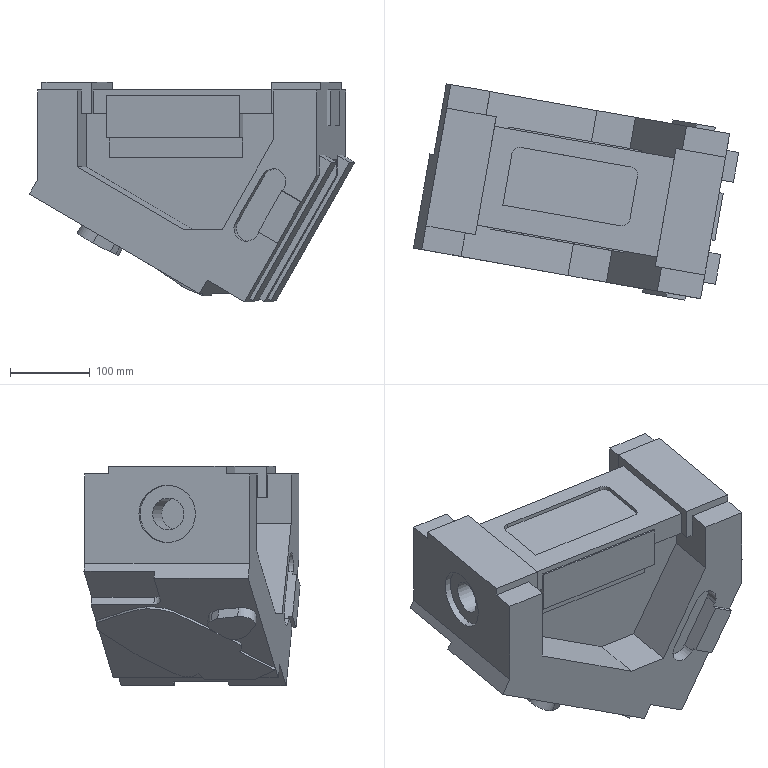Part | NX | features solid 2 | 1 solid | 123 faces | box 408 x 271.058 x 275.862 mm | volume 11212890 mm3 | plane 106 | cylinder 13 | spline 4 | commonest cylinder face diameters 20 x4 32 x4 30 x2 34 x1 40 x1 72 x1